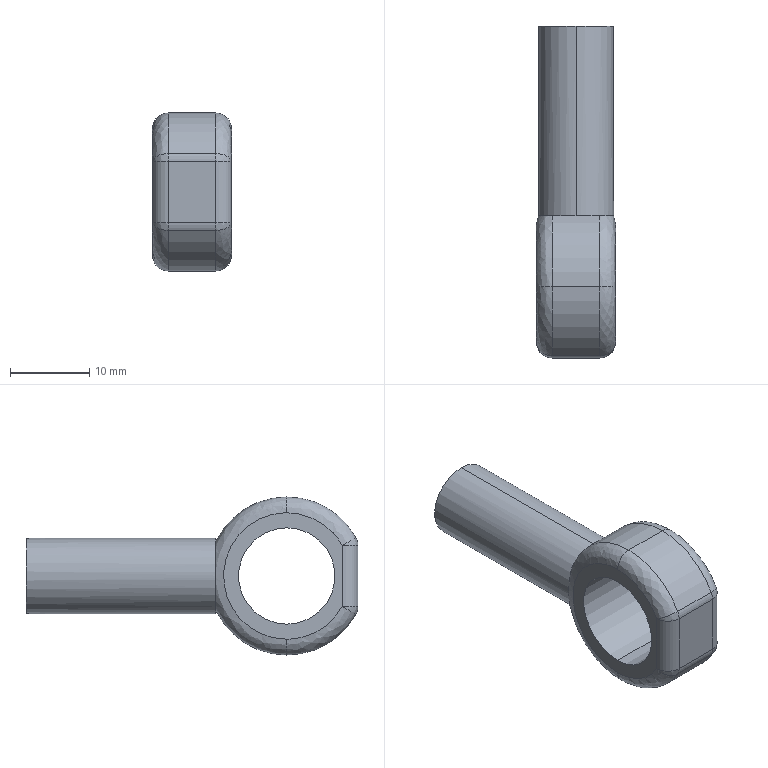Part | SolidWorks | features BaseBody 1 | 1 solid | 31 faces | box 10 x 42 x 20 mm | volume 3464 mm3 | cylinder 11 | spline 10 | plane 10 | commonest cylinder face diameters 4 x4 20 x3 9.5 x2 12.2 x2
STEP:
#1=CARTESIAN_POINT('',(5.,0.,8.));
#2=VERTEX_POINT('',#1);
#3=CARTESIAN_POINT('',(5.,-7.,3.873));
#4=VERTEX_POINT('',#3);
#5=CARTESIAN_POINT('',(5.,0.,8.));
#6=CARTESIAN_POINT('',(5.,-0.3506,8.));
#7=CARTESIAN_POINT('',(5.,-0.8722,7.966));
#8=CARTESIAN_POINT('',(5.,-1.473,7.867));
#9=CARTESIAN_POINT('',(5.,-1.771,7.802));
#10=CARTESIAN_POINT('',(5.,-1.899,7.771));
#11=CARTESIAN_POINT('',(5.,-1.984,7.75));
#12=CARTESIAN_POINT('',(5.,-2.025,7.74));
#13=CARTESIAN_POINT('',(5.,-2.771,7.54));
#14=CARTESIAN_POINT('',(5.,-3.437,7.261));
#15=CARTESIAN_POINT('',(5.,-4.376,6.707));
#16=CARTESIAN_POINT('',(5.,-4.823,6.401));
#17=CARTESIAN_POINT('',(5.,-5.305,5.993));
#18=CARTESIAN_POINT('',(5.,-5.536,5.776));
#19=CARTESIAN_POINT('',(5.,-5.633,5.681));
#20=CARTESIAN_POINT('',(5.,-5.697,5.617));
#21=CARTESIAN_POINT('',(5.,-5.73,5.583));
#22=CARTESIAN_POINT('',(5.,-6.247,5.046));
#23=CARTESIAN_POINT('',(5.,-6.66,4.487));
#24=CARTESIAN_POINT('',(5.,-7.,3.873));
#25=B_SPLINE_CURVE_WITH_KNOTS('',3,(#5,#6,#7,#8,#9,#10,#11,#12,#13,#14,#15,#16,#17,#18,#19,#20,#21,#22,#23,#24),.UNSPECIFIED.,.F.,.F.,(4,1,1,1,2,2,2,1,1,1,2,2,4),(0.,0.125,0.1875,0.2187,0.2344,0.25,0.5,0.625,0.6875,0.7187,0.7344,0.75,1.),.UNSPECIFIED.);
#26=EDGE_CURVE('',#2,#4,#25,.T.);
#27=ORIENTED_EDGE('',*,*,#26,.F.);
#28=CARTESIAN_POINT('',(3.,0.,10.));
#29=VERTEX_POINT('',#28);
#30=CARTESIAN_POINT('',(3.,0.,8.));
#31=DIRECTION('',(0.,-1.,0.));
#32=DIRECTION('',(0.,0.,1.));
#33=AXIS2_PLACEMENT_3D('',#30,#31,#32);
#34=CIRCLE('',#33,2.);
#35=EDGE_CURVE('',#2,#29,#34,.T.);
#36=ORIENTED_EDGE('',*,*,#35,.T.);
#37=CARTESIAN_POINT('',(3.,-8.75,4.841));
#38=VERTEX_POINT('',#37);
#39=CARTESIAN_POINT('',(3.,0.,0.));
#40=DIRECTION('',(1.,0.,0.));
#41=DIRECTION('',(0.,0.,-1.));
#42=AXIS2_PLACEMENT_3D('',#39,#40,#41);
#43=CIRCLE('',#42,10.);
#44=EDGE_CURVE('',#29,#38,#43,.T.);
#45=ORIENTED_EDGE('',*,*,#44,.T.);
#46=CARTESIAN_POINT('',(3.,-7.,3.873));
#47=DIRECTION('',(0.,0.4841,0.875));
#48=DIRECTION('',(0.,-0.875,0.4841));
#49=AXIS2_PLACEMENT_3D('',#46,#47,#48);
#50=CIRCLE('',#49,2.);
#51=EDGE_CURVE('',#38,#4,#50,.T.);
#52=ORIENTED_EDGE('',*,*,#51,.T.);
#53=EDGE_LOOP('',(#27,#36,#45,#52));
#54=FACE_OUTER_BOUND('',#53,.T.);
#55=CARTESIAN_POINT('',(5.,0.,8.));
#56=CARTESIAN_POINT('',(5.,-2.984,8.));
#57=CARTESIAN_POINT('',(5.,-5.555,6.484));
#58=CARTESIAN_POINT('',(5.,-7.,3.873));
#59=CARTESIAN_POINT('',(5.,0.,9.172));
#60=CARTESIAN_POINT('',(5.,-3.421,9.172));
#61=CARTESIAN_POINT('',(5.,-6.369,7.434));
#62=CARTESIAN_POINT('',(5.,-8.025,4.44));
#63=CARTESIAN_POINT('',(4.172,0.,10.));
#64=CARTESIAN_POINT('',(4.172,-3.73,10.));
#65=CARTESIAN_POINT('',(4.172,-6.944,8.105));
#66=CARTESIAN_POINT('',(4.172,-8.75,4.841));
#67=CARTESIAN_POINT('',(3.,0.,10.));
#68=CARTESIAN_POINT('',(3.,-3.73,10.));
#69=CARTESIAN_POINT('',(3.,-6.944,8.105));
#70=CARTESIAN_POINT('',(3.,-8.75,4.841));
#71=(BOUNDED_SURFACE()B_SPLINE_SURFACE(3,3,((#55,#56,#57,#58),(#59,#60,#61,#62),(#63,#64,#65,#66),(#67,#68,#69,#70)),.UNSPECIFIED.,.F.,.F.,.F.)B_SPLINE_SURFACE_WITH_KNOTS((4,4),(4,4),(0.,1.),(0.,1.),.UNSPECIFIED.)GEOMETRIC_REPRESENTATION_ITEM()RATIONAL_B_SPLINE_SURFACE(((1.,0.9076,0.9076,1.),(0.8047,0.7304,0.7304,0.8047),(0.8047,0.7304,0.7304,0.8047),(1.,0.9076,0.9076,1.)))REPRESENTATION_ITEM('')SURFACE());
#72=ADVANCED_FACE('',(#54),#71,.T.);
#73=ORIENTED_EDGE('',*,*,#35,.F.);
#74=CARTESIAN_POINT('',(5.,0.,-8.));
#75=VERTEX_POINT('',#74);
#76=CARTESIAN_POINT('',(5.,0.,8.));
#77=CARTESIAN_POINT('',(5.,16.,8.));
#78=CARTESIAN_POINT('',(5.,16.,-8.));
#79=CARTESIAN_POINT('',(5.,0.,-8.));
#80=(BOUNDED_CURVE()B_SPLINE_CURVE(3,(#76,#77,#78,#79),.UNSPECIFIED.,.F.,.T.)B_SPLINE_CURVE_WITH_KNOTS((4,4),(0.,1.),.UNSPECIFIED.)CURVE()GEOMETRIC_REPRESENTATION_ITEM()RATIONAL_B_SPLINE_CURVE((1.,0.3333,0.3333,1.))REPRESENTATION_ITEM(''));
#81=EDGE_CURVE('',#2,#75,#80,.T.);
#82=ORIENTED_EDGE('',*,*,#81,.T.);
#83=CARTESIAN_POINT('',(3.,0.,-10.));
#84=VERTEX_POINT('',#83);
#85=CARTESIAN_POINT('',(3.,0.,-8.));
#86=DIRECTION('',(0.,1.,0.));
#87=DIRECTION('',(0.,0.,-1.));
#88=AXIS2_PLACEMENT_3D('',#85,#86,#87);
#89=CIRCLE('',#88,2.);
#90=EDGE_CURVE('',#75,#84,#89,.T.);
#91=ORIENTED_EDGE('',*,*,#90,.T.);
#92=CARTESIAN_POINT('',(3.,9.,-4.359));
#93=VERTEX_POINT('',#92);
#94=CARTESIAN_POINT('',(3.,0.,0.));
#95=DIRECTION('',(-1.,0.,0.));
#96=DIRECTION('',(0.,0.,1.));
#97=AXIS2_PLACEMENT_3D('',#94,#95,#96);
#98=CIRCLE('',#97,10.);
#99=EDGE_CURVE('',#93,#84,#98,.T.);
#100=ORIENTED_EDGE('',*,*,#99,.F.);
#101=CARTESIAN_POINT('',(4.724,9.,-0.4952));
#102=VERTEX_POINT('',#101);
#103=CARTESIAN_POINT('',(3.,9.,-4.359));
#104=CARTESIAN_POINT('',(3.194,9.,-4.359));
#105=CARTESIAN_POINT('',(3.381,9.,-4.292));
#106=CARTESIAN_POINT('',(3.702,9.,-4.077));
#107=CARTESIAN_POINT('',(3.834,9.,-3.936));
#108=CARTESIAN_POINT('',(4.06,9.,-3.623));
#109=CARTESIAN_POINT('',(4.15,9.,-3.455));
#110=CARTESIAN_POINT('',(4.304,9.,-3.107));
#111=CARTESIAN_POINT('',(4.367,9.,-2.924));
#112=CARTESIAN_POINT('',(4.526,9.,-2.375));
#113=CARTESIAN_POINT('',(4.592,9.,-2.003));
#114=CARTESIAN_POINT('',(4.686,9.,-1.253));
#115=CARTESIAN_POINT('',(4.712,9.,-0.8754));
#116=CARTESIAN_POINT('',(4.724,9.,-0.4952));
#117=B_SPLINE_CURVE_WITH_KNOTS('',3,(#103,#104,#105,#106,#107,#108,#109,#110,#111,#112,#113,#114,#115,#116),.UNSPECIFIED.,.F.,.F.,(4,2,2,2,2,2,4),(0.,0.0005743,0.001149,0.001723,0.002297,0.003446,0.004594),.UNSPECIFIED.);
#118=EDGE_CURVE('',#93,#102,#117,.T.);
#119=ORIENTED_EDGE('',*,*,#118,.T.);
#120=CARTESIAN_POINT('',(4.724,9.,0.4952));
#121=VERTEX_POINT('',#120);
#122=CARTESIAN_POINT('',(4.724,9.,-0.4952));
#123=CARTESIAN_POINT('',(4.741,8.98,-0.3301));
#124=CARTESIAN_POINT('',(4.759,8.957,0.));
#125=CARTESIAN_POINT('',(4.741,8.98,0.3301));
#126=CARTESIAN_POINT('',(4.724,9.,0.4952));
#127=B_SPLINE_CURVE_WITH_KNOTS('',3,(#122,#123,#124,#125,#126),.UNSPECIFIED.,.F.,.F.,(4,1,4),(0.,0.0004952,0.0009903),.UNSPECIFIED.);
#128=EDGE_CURVE('',#102,#121,#127,.T.);
#129=ORIENTED_EDGE('',*,*,#128,.T.);
#130=CARTESIAN_POINT('',(3.,9.,4.359));
#131=VERTEX_POINT('',#130);
#132=CARTESIAN_POINT('',(4.724,9.,0.4952));
#133=CARTESIAN_POINT('',(4.712,9.,0.8759));
#134=CARTESIAN_POINT('',(4.686,9.,1.255));
#135=CARTESIAN_POINT('',(4.592,9.,2.008));
#136=CARTESIAN_POINT('',(4.524,9.,2.385));
#137=CARTESIAN_POINT('',(4.364,9.,2.934));
#138=CARTESIAN_POINT('',(4.301,9.,3.114));
#139=CARTESIAN_POINT('',(4.146,9.,3.462));
#140=CARTESIAN_POINT('',(4.056,9.,3.629));
#141=CARTESIAN_POINT('',(3.835,9.,3.936));
#142=CARTESIAN_POINT('',(3.701,9.,4.079));
#143=CARTESIAN_POINT('',(3.461,9.,4.239));
#144=CARTESIAN_POINT('',(3.374,9.,4.282));
#145=CARTESIAN_POINT('',(3.194,9.,4.342));
#146=CARTESIAN_POINT('',(3.097,9.,4.359));
#147=CARTESIAN_POINT('',(3.,9.,4.359));
#148=B_SPLINE_CURVE_WITH_KNOTS('',3,(#132,#133,#134,#135,#136,#137,#138,#139,#140,#141,#142,#143,#144,#145,#146,#147),.UNSPECIFIED.,.F.,.F.,(4,2,2,2,2,2,2,4),(0.,0.001139,0.002277,0.002846,0.003416,0.003985,0.00427,0.004554),.UNSPECIFIED.);
#149=EDGE_CURVE('',#121,#131,#148,.T.);
#150=ORIENTED_EDGE('',*,*,#149,.T.);
#151=CARTESIAN_POINT('',(3.,0.,0.));
#152=DIRECTION('',(1.,0.,0.));
#153=DIRECTION('',(0.,0.,-1.));
#154=AXIS2_PLACEMENT_3D('',#151,#152,#153);
#155=CIRCLE('',#154,10.);
#156=EDGE_CURVE('',#131,#29,#155,.T.);
#157=ORIENTED_EDGE('',*,*,#156,.T.);
#158=EDGE_LOOP('',(#73,#82,#91,#100,#119,#129,#150,#157));
#159=FACE_OUTER_BOUND('',#158,.T.);
#160=CARTESIAN_POINT('',(5.,0.,-8.));
#161=CARTESIAN_POINT('',(5.,16.,-8.));
#162=CARTESIAN_POINT('',(5.,16.,8.));
#163=CARTESIAN_POINT('',(5.,0.,8.));
#164=CARTESIAN_POINT('',(5.,0.,-9.172));
#165=CARTESIAN_POINT('',(5.,18.343,-9.172));
#166=CARTESIAN_POINT('',(5.,18.343,9.172));
#167=CARTESIAN_POINT('',(5.,0.,9.172));
#168=CARTESIAN_POINT('',(4.172,0.,-10.));
#169=CARTESIAN_POINT('',(4.172,20.,-10.));
#170=CARTESIAN_POINT('',(4.172,20.,10.));
#171=CARTESIAN_POINT('',(4.172,0.,10.));
#172=CARTESIAN_POINT('',(3.,0.,-10.));
#173=CARTESIAN_POINT('',(3.,20.,-10.));
#174=CARTESIAN_POINT('',(3.,20.,10.));
#175=CARTESIAN_POINT('',(3.,0.,10.));
#176=(BOUNDED_SURFACE()B_SPLINE_SURFACE(3,3,((#160,#161,#162,#163),(#164,#165,#166,#167),(#168,#169,#170,#171),(#172,#173,#174,#175)),.UNSPECIFIED.,.F.,.F.,.F.)B_SPLINE_SURFACE_WITH_KNOTS((4,4),(4,4),(0.,1.),(0.,1.),.UNSPECIFIED.)GEOMETRIC_REPRESENTATION_ITEM()RATIONAL_B_SPLINE_SURFACE(((1.,0.3333,0.3333,1.),(0.8047,0.2682,0.2682,0.8047),(0.8047,0.2682,0.2682,0.8047),(1.,0.3333,0.3333,1.)))REPRESENTATION_ITEM('')SURFACE());
#177=ADVANCED_FACE('',(#159),#176,.T.);
#178=CARTESIAN_POINT('',(-3.,0.,10.));
#179=VERTEX_POINT('',#178);
#180=CARTESIAN_POINT('',(-3.,-8.75,4.841));
#181=VERTEX_POINT('',#180);
#182=CARTESIAN_POINT('',(-3.,0.,0.));
#183=DIRECTION('',(1.,0.,0.));
#184=DIRECTION('',(0.,0.,1.));
#185=AXIS2_PLACEMENT_3D('',#182,#183,#184);
#186=CIRCLE('',#185,10.);
#187=EDGE_CURVE('',#179,#181,#186,.T.);
#188=ORIENTED_EDGE('',*,*,#187,.F.);
#189=CARTESIAN_POINT('',(-5.,0.,8.));
#190=VERTEX_POINT('',#189);
#191=CARTESIAN_POINT('',(-3.,0.,8.));
#192=DIRECTION('',(0.,-1.,0.));
#193=DIRECTION('',(0.,0.,1.));
#194=AXIS2_PLACEMENT_3D('',#191,#192,#193);
#195=CIRCLE('',#194,2.);
#196=EDGE_CURVE('',#179,#190,#195,.T.);
#197=ORIENTED_EDGE('',*,*,#196,.T.);
#198=CARTESIAN_POINT('',(-5.,-7.,3.873));
#199=VERTEX_POINT('',#198);
#200=CARTESIAN_POINT('',(-5.,0.,8.));
#201=CARTESIAN_POINT('',(-5.,-2.984,8.));
#202=CARTESIAN_POINT('',(-5.,-5.555,6.484));
#203=CARTESIAN_POINT('',(-5.,-7.,3.873));
#204=(BOUNDED_CURVE()B_SPLINE_CURVE(3,(#200,#201,#202,#203),.UNSPECIFIED.,.F.,.F.)B_SPLINE_CURVE_WITH_KNOTS((4,4),(0.,1.),.UNSPECIFIED.)CURVE()GEOMETRIC_REPRESENTATION_ITEM()RATIONAL_B_SPLINE_CURVE((1.,0.9076,0.9076,1.))REPRESENTATION_ITEM(''));
#205=EDGE_CURVE('',#190,#199,#204,.T.);
#206=ORIENTED_EDGE('',*,*,#205,.T.);
#207=CARTESIAN_POINT('',(-3.,-7.,3.873));
#208=DIRECTION('',(0.,0.4841,0.875));
#209=DIRECTION('',(0.,-0.875,0.4841));
#210=AXIS2_PLACEMENT_3D('',#207,#208,#209);
#211=CIRCLE('',#210,2.);
#212=EDGE_CURVE('',#199,#181,#211,.T.);
#213=ORIENTED_EDGE('',*,*,#212,.T.);
#214=EDGE_LOOP('',(#188,#197,#206,#213));
#215=FACE_OUTER_BOUND('',#214,.T.);
#216=CARTESIAN_POINT('',(-3.,0.,10.));
#217=CARTESIAN_POINT('',(-3.,-3.73,10.));
#218=CARTESIAN_POINT('',(-3.,-6.944,8.105));
#219=CARTESIAN_POINT('',(-3.,-8.75,4.841));
#220=CARTESIAN_POINT('',(-4.172,0.,10.));
#221=CARTESIAN_POINT('',(-4.172,-3.73,10.));
#222=CARTESIAN_POINT('',(-4.172,-6.944,8.105));
#223=CARTESIAN_POINT('',(-4.172,-8.75,4.841));
#224=CARTESIAN_POINT('',(-5.,0.,9.172));
#225=CARTESIAN_POINT('',(-5.,-3.421,9.172));
#226=CARTESIAN_POINT('',(-5.,-6.369,7.434));
#227=CARTESIAN_POINT('',(-5.,-8.025,4.44));
#228=CARTESIAN_POINT('',(-5.,0.,8.));
#229=CARTESIAN_POINT('',(-5.,-2.984,8.));
#230=CARTESIAN_POINT('',(-5.,-5.555,6.484));
#231=CARTESIAN_POINT('',(-5.,-7.,3.873));
#232=(BOUNDED_SURFACE()B_SPLINE_SURFACE(3,3,((#216,#217,#218,#219),(#220,#221,#222,#223),(#224,#225,#226,#227),(#228,#229,#230,#231)),.UNSPECIFIED.,.F.,.F.,.F.)B_SPLINE_SURFACE_WITH_KNOTS((4,4),(4,4),(0.,1.),(0.,1.),.UNSPECIFIED.)GEOMETRIC_REPRESENTATION_ITEM()RATIONAL_B_SPLINE_SURFACE(((1.,0.9076,0.9076,1.),(0.8047,0.7304,0.7304,0.8047),(0.8047,0.7304,0.7304,0.8047),(1.,0.9076,0.9076,1.)))REPRESENTATION_ITEM('')SURFACE());
#233=ADVANCED_FACE('',(#215),#232,.T.);
#234=ORIENTED_EDGE('',*,*,#196,.F.);
#235=CARTESIAN_POINT('',(-3.,9.,4.359));
#236=VERTEX_POINT('',#235);
#237=CARTESIAN_POINT('',(-3.,0.,0.));
#238=DIRECTION('',(1.,0.,0.));
#239=DIRECTION('',(0.,0.,1.));
#240=AXIS2_PLACEMENT_3D('',#237,#238,#239);
#241=CIRCLE('',#240,10.);
#242=EDGE_CURVE('',#236,#179,#241,.T.);
#243=ORIENTED_EDGE('',*,*,#242,.F.);
#244=CARTESIAN_POINT('',(-4.724,9.,0.4952));
#245=VERTEX_POINT('',#244);
#246=CARTESIAN_POINT('',(-3.,9.,4.359));
#247=CARTESIAN_POINT('',(-3.194,9.,4.359));
#248=CARTESIAN_POINT('',(-3.381,9.,4.292));
#249=CARTESIAN_POINT('',(-3.702,9.,4.077));
#250=CARTESIAN_POINT('',(-3.834,9.,3.936));
#251=CARTESIAN_POINT('',(-4.06,9.,3.623));
#252=CARTESIAN_POINT('',(-4.15,9.,3.455));
#253=CARTESIAN_POINT('',(-4.304,9.,3.107));
#254=CARTESIAN_POINT('',(-4.367,9.,2.924));
#255=CARTESIAN_POINT('',(-4.526,9.,2.375));
#256=CARTESIAN_POINT('',(-4.592,9.,2.003));
#257=CARTESIAN_POINT('',(-4.686,9.,1.253));
#258=CARTESIAN_POINT('',(-4.712,9.,0.8754));
#259=CARTESIAN_POINT('',(-4.724,9.,0.4952));
#260=B_SPLINE_CURVE_WITH_KNOTS('',3,(#246,#247,#248,#249,#250,#251,#252,#253,#254,#255,#256,#257,#258,#259),.UNSPECIFIED.,.F.,.F.,(4,2,2,2,2,2,4),(0.,0.0005743,0.001149,0.001723,0.002297,0.003446,0.004594),.UNSPECIFIED.);
#261=EDGE_CURVE('',#236,#245,#260,.T.);
#262=ORIENTED_EDGE('',*,*,#261,.T.);
#263=CARTESIAN_POINT('',(-4.724,9.,-0.4952));
#264=VERTEX_POINT('',#263);
#265=CARTESIAN_POINT('',(-4.724,9.,0.4952));
#266=CARTESIAN_POINT('',(-4.741,8.98,0.3301));
#267=CARTESIAN_POINT('',(-4.759,8.957,0.));
#268=CARTESIAN_POINT('',(-4.741,8.98,-0.3301));
#269=CARTESIAN_POINT('',(-4.724,9.,-0.4952));
#270=B_SPLINE_CURVE_WITH_KNOTS('',3,(#265,#266,#267,#268,#269),.UNSPECIFIED.,.F.,.F.,(4,1,4),(0.,0.0004952,0.0009903),.UNSPECIFIED.);
#271=EDGE_CURVE('',#245,#264,#270,.T.);
#272=ORIENTED_EDGE('',*,*,#271,.T.);
#273=CARTESIAN_POINT('',(-3.,9.,-4.359));
#274=VERTEX_POINT('',#273);
#275=CARTESIAN_POINT('',(-4.724,9.,-0.4952));
#276=CARTESIAN_POINT('',(-4.712,9.,-0.8759));
#277=CARTESIAN_POINT('',(-4.686,9.,-1.255));
#278=CARTESIAN_POINT('',(-4.592,9.,-2.008));
#279=CARTESIAN_POINT('',(-4.524,9.,-2.385));
#280=CARTESIAN_POINT('',(-4.364,9.,-2.934));
#281=CARTESIAN_POINT('',(-4.301,9.,-3.114));
#282=CARTESIAN_POINT('',(-4.146,9.,-3.462));
#283=CARTESIAN_POINT('',(-4.056,9.,-3.629));
#284=CARTESIAN_POINT('',(-3.835,9.,-3.936));
#285=CARTESIAN_POINT('',(-3.701,9.,-4.079));
#286=CARTESIAN_POINT('',(-3.461,9.,-4.239));
#287=CARTESIAN_POINT('',(-3.374,9.,-4.282));
#288=CARTESIAN_POINT('',(-3.194,9.,-4.342));
#289=CARTESIAN_POINT('',(-3.097,9.,-4.359));
#290=CARTESIAN_POINT('',(-3.,9.,-4.359));
#291=B_SPLINE_CURVE_WITH_KNOTS('',3,(#275,#276,#277,#278,#279,#280,#281,#282,#283,#284,#285,#286,#287,#288,#289,#290),.UNSPECIFIED.,.F.,.F.,(4,2,2,2,2,2,2,4),(0.,0.001139,0.002277,0.002846,0.003416,0.003985,0.00427,0.004554),.UNSPECIFIED.);
#292=EDGE_CURVE('',#264,#274,#291,.T.);
#293=ORIENTED_EDGE('',*,*,#292,.T.);
#294=CARTESIAN_POINT('',(-3.,0.,-10.));
#295=VERTEX_POINT('',#294);
#296=CARTESIAN_POINT('',(-3.,0.,0.));
#297=DIRECTION('',(1.,0.,0.));
#298=DIRECTION('',(0.,0.,1.));
#299=AXIS2_PLACEMENT_3D('',#296,#297,#298);
#300=CIRCLE('',#299,10.);
#301=EDGE_CURVE('',#295,#274,#300,.T.);
#302=ORIENTED_EDGE('',*,*,#301,.F.);
#303=CARTESIAN_POINT('',(-5.,0.,-8.));
#304=VERTEX_POINT('',#303);
#305=CARTESIAN_POINT('',(-3.,0.,-8.));
#306=DIRECTION('',(0.,1.,0.));
#307=DIRECTION('',(0.,0.,-1.));
#308=AXIS2_PLACEMENT_3D('',#305,#306,#307);
#309=CIRCLE('',#308,2.);
#310=EDGE_CURVE('',#295,#304,#309,.T.);
#311=ORIENTED_EDGE('',*,*,#310,.T.);
#312=CARTESIAN_POINT('',(-5.,0.,-8.));
#313=CARTESIAN_POINT('',(-5.,16.,-8.));
#314=CARTESIAN_POINT('',(-5.,16.,8.));
#315=CARTESIAN_POINT('',(-5.,0.,8.));
#316=(BOUNDED_CURVE()B_SPLINE_CURVE(3,(#312,#313,#314,#315),.UNSPECIFIED.,.F.,.F.)B_SPLINE_CURVE_WITH_KNOTS((4,4),(0.,1.),.UNSPECIFIED.)CURVE()GEOMETRIC_REPRESENTATION_ITEM()RATIONAL_B_SPLINE_CURVE((1.,0.3333,0.3333,1.))REPRESENTATION_ITEM(''));
#317=EDGE_CURVE('',#304,#190,#316,.T.);
#318=ORIENTED_EDGE('',*,*,#317,.T.);
#319=EDGE_LOOP('',(#234,#243,#262,#272,#293,#302,#311,#318));
#320=FACE_OUTER_BOUND('',#319,.T.);
#321=CARTESIAN_POINT('',(-3.,0.,-10.));
#322=CARTESIAN_POINT('',(-3.,20.,-10.));
#323=CARTESIAN_POINT('',(-3.,20.,10.));
#324=CARTESIAN_POINT('',(-3.,0.,10.));
#325=CARTESIAN_POINT('',(-4.172,0.,-10.));
#326=CARTESIAN_POINT('',(-4.172,20.,-10.));
#327=CARTESIAN_POINT('',(-4.172,20.,10.));
#328=CARTESIAN_POINT('',(-4.172,0.,10.));
#329=CARTESIAN_POINT('',(-5.,0.,-9.172));
#330=CARTESIAN_POINT('',(-5.,18.343,-9.172));
#331=CARTESIAN_POINT('',(-5.,18.343,9.172));
#332=CARTESIAN_POINT('',(-5.,0.,9.172));
#333=CARTESIAN_POINT('',(-5.,0.,-8.));
#334=CARTESIAN_POINT('',(-5.,16.,-8.));
#335=CARTESIAN_POINT('',(-5.,16.,8.));
#336=CARTESIAN_POINT('',(-5.,0.,8.));
#337=(BOUNDED_SURFACE()B_SPLINE_SURFACE(3,3,((#321,#322,#323,#324),(#325,#326,#327,#328),(#329,#330,#331,#332),(#333,#334,#335,#336)),.UNSPECIFIED.,.F.,.F.,.T.)B_SPLINE_SURFACE_WITH_KNOTS((4,4),(4,4),(0.,1.),(0.,1.),.UNSPECIFIED.)GEOMETRIC_REPRESENTATION_ITEM()RATIONAL_B_SPLINE_SURFACE(((1.,0.3333,0.3333,1.),(0.8047,0.2682,0.2682,0.8047),(0.8047,0.2682,0.2682,0.8047),(1.,0.3333,0.3333,1.)))REPRESENTATION_ITEM('')SURFACE());
#338=ADVANCED_FACE('',(#320),#337,.T.);
#339=CARTESIAN_POINT('',(0.,33.,-4.75));
#340=VERTEX_POINT('',#339);
#341=CARTESIAN_POINT('',(0.,33.,4.75));
#342=VERTEX_POINT('',#341);
#343=CARTESIAN_POINT('',(0.,33.,0.));
#344=DIRECTION('',(0.,-1.,0.));
#345=DIRECTION('',(0.,0.,-1.));
#346=AXIS2_PLACEMENT_3D('',#343,#344,#345);
#347=CIRCLE('',#346,4.75);
#348=EDGE_CURVE('',#340,#342,#347,.T.);
#349=ORIENTED_EDGE('',*,*,#348,.T.);
#350=CARTESIAN_POINT('',(0.,9.,4.75));
#351=VERTEX_POINT('',#350);
#352=CARTESIAN_POINT('',(0.,33.,4.75));
#353=DIRECTION('',(0.,-1.,0.));
#354=VECTOR('',#353,1000.);
#355=LINE('',#352,#354);
#356=EDGE_CURVE('',#342,#351,#355,.T.);
#357=ORIENTED_EDGE('',*,*,#356,.T.);
#358=CARTESIAN_POINT('',(1.887,9.,4.359));
#359=VERTEX_POINT('',#358);
#360=CARTESIAN_POINT('',(0.,9.,0.));
#361=DIRECTION('',(0.,1.,0.));
#362=DIRECTION('',(0.,0.,-1.));
#363=AXIS2_PLACEMENT_3D('',#360,#361,#362);
#364=CIRCLE('',#363,4.75);
#365=EDGE_CURVE('',#351,#359,#364,.T.);
#366=ORIENTED_EDGE('',*,*,#365,.T.);
#367=CARTESIAN_POINT('',(0.,9.,0.));
#368=DIRECTION('',(0.,1.,0.));
#369=DIRECTION('',(0.,0.,-1.));
#370=AXIS2_PLACEMENT_3D('',#367,#368,#369);
#371=CIRCLE('',#370,4.75);
#372=EDGE_CURVE('',#359,#121,#371,.T.);
#373=ORIENTED_EDGE('',*,*,#372,.T.);
#374=ORIENTED_EDGE('',*,*,#128,.F.);
#375=CARTESIAN_POINT('',(1.887,9.,-4.359));
#376=VERTEX_POINT('',#375);
#377=CARTESIAN_POINT('',(0.,9.,0.));
#378=DIRECTION('',(0.,1.,0.));
#379=DIRECTION('',(0.,0.,-1.));
#380=AXIS2_PLACEMENT_3D('',#377,#378,#379);
#381=CIRCLE('',#380,4.75);
#382=EDGE_CURVE('',#102,#376,#381,.T.);
#383=ORIENTED_EDGE('',*,*,#382,.T.);
#384=CARTESIAN_POINT('',(0.,9.,-4.75));
#385=VERTEX_POINT('',#384);
#386=CARTESIAN_POINT('',(0.,9.,0.));
#387=DIRECTION('',(0.,1.,0.));
#388=DIRECTION('',(0.,0.,-1.));
#389=AXIS2_PLACEMENT_3D('',#386,#387,#388);
#390=CIRCLE('',#389,4.75);
#391=EDGE_CURVE('',#376,#385,#390,.T.);
#392=ORIENTED_EDGE('',*,*,#391,.T.);
#393=CARTESIAN_POINT('',(0.,33.,-4.75));
#394=DIRECTION('',(0.,-1.,0.));
#395=VECTOR('',#394,1000.);
#396=LINE('',#393,#395);
#397=EDGE_CURVE('',#340,#385,#396,.T.);
#398=ORIENTED_EDGE('',*,*,#397,.F.);
#399=EDGE_LOOP('',(#349,#357,#366,#373,#374,#383,#392,#398));
#400=FACE_OUTER_BOUND('',#399,.T.);
#401=CARTESIAN_POINT('',(0.,33.,0.));
#402=DIRECTION('',(0.,-1.,0.));
#403=DIRECTION('',(0.,0.,-1.));
#404=AXIS2_PLACEMENT_3D('',#401,#402,#403);
#405=CYLINDRICAL_SURFACE('',#404,4.75);
#406=ADVANCED_FACE('',(#400),#405,.T.);
#407=ORIENTED_EDGE('',*,*,#44,.F.);
#408=CARTESIAN_POINT('',(5.,0.,10.));
#409=DIRECTION('',(-1.,0.,0.));
#410=VECTOR('',#409,1000.);
#411=LINE('',#408,#410);
#412=EDGE_CURVE('',#29,#179,#411,.T.);
#413=ORIENTED_EDGE('',*,*,#412,.T.);
#414=ORIENTED_EDGE('',*,*,#187,.T.);
#415=CARTESIAN_POINT('',(5.,-8.75,4.841));
#416=DIRECTION('',(1.,0.,0.));
#417=VECTOR('',#416,1000.);
#418=LINE('',#415,#417);
#419=EDGE_CURVE('',#181,#38,#418,.T.);
#420=ORIENTED_EDGE('',*,*,#419,.T.);
#421=EDGE_LOOP('',(#407,#413,#414,#420));
#422=FACE_OUTER_BOUND('',#421,.T.);
#423=CARTESIAN_POINT('',(5.,0.,0.));
#424=DIRECTION('',(-1.,0.,0.));
#425=DIRECTION('',(0.,0.,1.));
#426=AXIS2_PLACEMENT_3D('',#423,#424,#425);
#427=CYLINDRICAL_SURFACE('',#426,10.);
#428=ADVANCED_FACE('',(#422),#427,.T.);
#429=CARTESIAN_POINT('',(5.,0.,-6.1));
#430=VERTEX_POINT('',#429);
#431=CARTESIAN_POINT('',(5.,0.,6.1));
#432=VERTEX_POINT('',#431);
#433=CARTESIAN_POINT('',(5.,0.,0.));
#434=DIRECTION('',(-1.,0.,0.));
#435=DIRECTION('',(0.,0.,1.));
#436=AXIS2_PLACEMENT_3D('',#433,#434,#435);
#437=CIRCLE('',#436,6.1);
#438=EDGE_CURVE('',#430,#432,#437,.T.);
#439=ORIENTED_EDGE('',*,*,#438,.F.);
#440=CARTESIAN_POINT('',(-5.,0.,-6.1));
#441=VERTEX_POINT('',#440);
#442=CARTESIAN_POINT('',(5.,0.,-6.1));
#443=DIRECTION('',(-1.,0.,0.));
#444=VECTOR('',#443,1000.);
#445=LINE('',#442,#444);
#446=EDGE_CURVE('',#430,#441,#445,.T.);
#447=ORIENTED_EDGE('',*,*,#446,.T.);
#448=CARTESIAN_POINT('',(-5.,0.,6.1));
#449=VERTEX_POINT('',#448);
#450=CARTESIAN_POINT('',(-5.,0.,0.));
#451=DIRECTION('',(-1.,0.,0.));
#452=DIRECTION('',(0.,0.,1.));
#453=AXIS2_PLACEMENT_3D('',#450,#451,#452);
#454=CIRCLE('',#453,6.1);
#455=EDGE_CURVE('',#441,#449,#454,.T.);
#456=ORIENTED_EDGE('',*,*,#455,.T.);
#457=CARTESIAN_POINT('',(5.,0.,6.1));
#458=DIRECTION('',(-1.,0.,0.));
#459=VECTOR('',#458,1000.);
#460=LINE('',#457,#459);
#461=EDGE_CURVE('',#432,#449,#460,.T.);
#462=ORIENTED_EDGE('',*,*,#461,.F.);
#463=EDGE_LOOP('',(#439,#447,#456,#462));
#464=FACE_OUTER_BOUND('',#463,.T.);
#465=CARTESIAN_POINT('',(5.,0.,0.));
#466=DIRECTION('',(-1.,0.,0.));
#467=DIRECTION('',(0.,0.,1.));
#468=AXIS2_PLACEMENT_3D('',#465,#466,#467);
#469=CYLINDRICAL_SURFACE('',#468,6.1);
#470=ADVANCED_FACE('',(#464),#469,.F.);
#471=ORIENTED_EDGE('',*,*,#356,.F.);
#472=CARTESIAN_POINT('',(0.,33.,0.));
#473=DIRECTION('',(0.,-1.,0.));
#474=DIRECTION('',(0.,0.,-1.));
#475=AXIS2_PLACEMENT_3D('',#472,#473,#474);
#476=CIRCLE('',#475,4.75);
#477=EDGE_CURVE('',#342,#340,#476,.T.);
#478=ORIENTED_EDGE('',*,*,#477,.T.);
#479=ORIENTED_EDGE('',*,*,#397,.T.);
#480=CARTESIAN_POINT('',(-1.887,9.,-4.359));
#481=VERTEX_POINT('',#480);
#482=CARTESIAN_POINT('',(0.,9.,0.));
#483=DIRECTION('',(0.,1.,0.));
#484=DIRECTION('',(0.,0.,-1.));
#485=AXIS2_PLACEMENT_3D('',#482,#483,#484);
#486=CIRCLE('',#485,4.75);
#487=EDGE_CURVE('',#385,#481,#486,.T.);
#488=ORIENTED_EDGE('',*,*,#487,.T.);
#489=CARTESIAN_POINT('',(0.,9.,0.));
#490=DIRECTION('',(0.,1.,0.));
#491=DIRECTION('',(0.,0.,-1.));
#492=AXIS2_PLACEMENT_3D('',#489,#490,#491);
#493=CIRCLE('',#492,4.75);
#494=EDGE_CURVE('',#481,#264,#493,.T.);
#495=ORIENTED_EDGE('',*,*,#494,.T.);
#496=ORIENTED_EDGE('',*,*,#271,.F.);
#497=CARTESIAN_POINT('',(-1.887,9.,4.359));
#498=VERTEX_POINT('',#497);
#499=CARTESIAN_POINT('',(0.,9.,0.));
#500=DIRECTION('',(0.,1.,0.));
#501=DIRECTION('',(0.,0.,-1.));
#502=AXIS2_PLACEMENT_3D('',#499,#500,#501);
#503=CIRCLE('',#502,4.75);
#504=EDGE_CURVE('',#245,#498,#503,.T.);
#505=ORIENTED_EDGE('',*,*,#504,.T.);
#506=CARTESIAN_POINT('',(0.,9.,0.));
#507=DIRECTION('',(0.,1.,0.));
#508=DIRECTION('',(0.,0.,-1.));
#509=AXIS2_PLACEMENT_3D('',#506,#507,#508);
#510=CIRCLE('',#509,4.75);
#511=EDGE_CURVE('',#498,#351,#510,.T.);
#512=ORIENTED_EDGE('',*,*,#511,.T.);
#513=EDGE_LOOP('',(#471,#478,#479,#488,#495,#496,#505,#512));
#514=FACE_OUTER_BOUND('',#513,.T.);
#515=CARTESIAN_POINT('',(0.,33.,0.));
#516=DIRECTION('',(0.,-1.,0.));
#517=DIRECTION('',(0.,0.,-1.));
#518=AXIS2_PLACEMENT_3D('',#515,#516,#517);
#519=CYLINDRICAL_SURFACE('',#518,4.75);
#520=ADVANCED_FACE('',(#514),#519,.T.);
#521=CARTESIAN_POINT('',(0.,9.,-4.359));
#522=DIRECTION('',(1.,0.,0.));
#523=VECTOR('',#522,1000.);
#524=LINE('',#521,#523);
#525=EDGE_CURVE('',#481,#376,#524,.T.);
#526=ORIENTED_EDGE('',*,*,#525,.F.);
#527=ORIENTED_EDGE('',*,*,#487,.F.);
#528=ORIENTED_EDGE('',*,*,#391,.F.);
#529=EDGE_LOOP('',(#526,#527,#528));
#530=FACE_OUTER_BOUND('',#529,.T.);
#531=CARTESIAN_POINT('',(0.,9.,0.));
#532=DIRECTION('',(0.,1.,0.));
#533=DIRECTION('',(0.,0.,1.));
#534=AXIS2_PLACEMENT_3D('',#531,#532,#533);
#535=PLANE('',#534);
#536=ADVANCED_FACE('',(#530),#535,.F.);
#537=ORIENTED_EDGE('',*,*,#118,.F.);
#538=CARTESIAN_POINT('',(5.,9.,-4.359));
#539=DIRECTION('',(1.,0.,0.));
#540=VECTOR('',#539,1000.);
#541=LINE('',#538,#540);
#542=EDGE_CURVE('',#376,#93,#541,.T.);
#543=ORIENTED_EDGE('',*,*,#542,.F.);
#544=ORIENTED_EDGE('',*,*,#382,.F.);
#545=EDGE_LOOP('',(#537,#543,#544));
#546=FACE_OUTER_BOUND('',#545,.T.);
#547=CARTESIAN_POINT('',(5.,9.,4.359));
#548=DIRECTION('',(0.,-1.,0.));
#549=DIRECTION('',(0.,0.,-1.));
#550=AXIS2_PLACEMENT_3D('',#547,#548,#549);
#551=PLANE('',#550);
#552=ADVANCED_FACE('',(#546),#551,.F.);
#553=CARTESIAN_POINT('',(5.,9.,4.359));
#554=DIRECTION('',(-1.,0.,0.));
#555=VECTOR('',#554,1000.);
#556=LINE('',#553,#555);
#557=EDGE_CURVE('',#131,#359,#556,.T.);
#558=ORIENTED_EDGE('',*,*,#557,.F.);
#559=ORIENTED_EDGE('',*,*,#149,.F.);
#560=ORIENTED_EDGE('',*,*,#372,.F.);
#561=EDGE_LOOP('',(#558,#559,#560));
#562=FACE_OUTER_BOUND('',#561,.T.);
#563=CARTESIAN_POINT('',(5.,9.,4.359));
#564=DIRECTION('',(0.,-1.,0.));
#565=DIRECTION('',(0.,0.,-1.));
#566=AXIS2_PLACEMENT_3D('',#563,#564,#565);
#567=PLANE('',#566);
#568=ADVANCED_FACE('',(#562),#567,.F.);
#569=CARTESIAN_POINT('',(0.,9.,4.359));
#570=DIRECTION('',(-1.,0.,0.));
#571=VECTOR('',#570,1000.);
#572=LINE('',#569,#571);
#573=EDGE_CURVE('',#359,#498,#572,.T.);
#574=ORIENTED_EDGE('',*,*,#573,.F.);
#575=ORIENTED_EDGE('',*,*,#365,.F.);
#576=ORIENTED_EDGE('',*,*,#511,.F.);
#577=EDGE_LOOP('',(#574,#575,#576));
#578=FACE_OUTER_BOUND('',#577,.T.);
#579=CARTESIAN_POINT('',(0.,9.,0.));
#580=DIRECTION('',(0.,1.,0.));
#581=DIRECTION('',(0.,0.,1.));
#582=AXIS2_PLACEMENT_3D('',#579,#580,#581);
#583=PLANE('',#582);
#584=ADVANCED_FACE('',(#578),#583,.F.);
#585=ORIENTED_EDGE('',*,*,#348,.F.);
#586=ORIENTED_EDGE('',*,*,#477,.F.);
#587=EDGE_LOOP('',(#585,#586));
#588=FACE_OUTER_BOUND('',#587,.T.);
#589=CARTESIAN_POINT('',(0.,33.,0.));
#590=DIRECTION('',(0.,1.,0.));
#591=DIRECTION('',(0.,0.,1.));
#592=AXIS2_PLACEMENT_3D('',#589,#590,#591);
#593=PLANE('',#592);
#594=ADVANCED_FACE('',(#588),#593,.T.);
#595=ORIENTED_EDGE('',*,*,#261,.F.);
#596=CARTESIAN_POINT('',(5.,9.,4.359));
#597=DIRECTION('',(-1.,0.,0.));
#598=VECTOR('',#597,1000.);
#599=LINE('',#596,#598);
#600=EDGE_CURVE('',#498,#236,#599,.T.);
#601=ORIENTED_EDGE('',*,*,#600,.F.);
#602=ORIENTED_EDGE('',*,*,#504,.F.);
#603=EDGE_LOOP('',(#595,#601,#602));
#604=FACE_OUTER_BOUND('',#603,.T.);
#605=CARTESIAN_POINT('',(5.,9.,4.359));
#606=DIRECTION('',(0.,-1.,0.));
#607=DIRECTION('',(0.,0.,-1.));
#608=AXIS2_PLACEMENT_3D('',#605,#606,#607);
#609=PLANE('',#608);
#610=ADVANCED_FACE('',(#604),#609,.F.);
#611=CARTESIAN_POINT('',(5.,9.,-4.359));
#612=DIRECTION('',(1.,0.,0.));
#613=VECTOR('',#612,1000.);
#614=LINE('',#611,#613);
#615=EDGE_CURVE('',#274,#481,#614,.T.);
#616=ORIENTED_EDGE('',*,*,#615,.F.);
#617=ORIENTED_EDGE('',*,*,#292,.F.);
#618=ORIENTED_EDGE('',*,*,#494,.F.);
#619=EDGE_LOOP('',(#616,#617,#618));
#620=FACE_OUTER_BOUND('',#619,.T.);
#621=CARTESIAN_POINT('',(5.,9.,4.359));
#622=DIRECTION('',(0.,-1.,0.));
#623=DIRECTION('',(0.,0.,-1.));
#624=AXIS2_PLACEMENT_3D('',#621,#622,#623);
#625=PLANE('',#624);
#626=ADVANCED_FACE('',(#620),#625,.F.);
#627=ORIENTED_EDGE('',*,*,#525,.T.);
#628=ORIENTED_EDGE('',*,*,#542,.T.);
#629=ORIENTED_EDGE('',*,*,#99,.T.);
#630=CARTESIAN_POINT('',(3.,-8.75,-4.841));
#631=VERTEX_POINT('',#630);
#632=CARTESIAN_POINT('',(3.,0.,0.));
#633=DIRECTION('',(-1.,0.,0.));
#634=DIRECTION('',(0.,0.,1.));
#635=AXIS2_PLACEMENT_3D('',#632,#633,#634);
#636=CIRCLE('',#635,10.);
#637=EDGE_CURVE('',#84,#631,#636,.T.);
#638=ORIENTED_EDGE('',*,*,#637,.T.);
#639=CARTESIAN_POINT('',(-3.,-8.75,-4.841));
#640=VERTEX_POINT('',#639);
#641=CARTESIAN_POINT('',(5.,-8.75,-4.841));
#642=DIRECTION('',(-1.,0.,0.));
#643=VECTOR('',#642,1000.);
#644=LINE('',#641,#643);
#645=EDGE_CURVE('',#631,#640,#644,.T.);
#646=ORIENTED_EDGE('',*,*,#645,.T.);
#647=CARTESIAN_POINT('',(-3.,0.,0.));
#648=DIRECTION('',(1.,0.,0.));
#649=DIRECTION('',(0.,0.,1.));
#650=AXIS2_PLACEMENT_3D('',#647,#648,#649);
#651=CIRCLE('',#650,10.);
#652=EDGE_CURVE('',#640,#295,#651,.T.);
#653=ORIENTED_EDGE('',*,*,#652,.T.);
#654=ORIENTED_EDGE('',*,*,#301,.T.);
#655=ORIENTED_EDGE('',*,*,#615,.T.);
#656=EDGE_LOOP('',(#627,#628,#629,#638,#646,#653,#654,#655));
#657=FACE_OUTER_BOUND('',#656,.T.);
#658=CARTESIAN_POINT('',(5.,0.,0.));
#659=DIRECTION('',(-1.,0.,0.));
#660=DIRECTION('',(0.,0.,1.));
#661=AXIS2_PLACEMENT_3D('',#658,#659,#660);
#662=CYLINDRICAL_SURFACE('',#661,10.);
#663=ADVANCED_FACE('',(#657),#662,.T.);
#664=ORIENTED_EDGE('',*,*,#90,.F.);
#665=CARTESIAN_POINT('',(5.,-7.,-3.873));
#666=VERTEX_POINT('',#665);
#667=CARTESIAN_POINT('',(5.,0.,-8.));
#668=CARTESIAN_POINT('',(5.,-2.984,-8.));
#669=CARTESIAN_POINT('',(5.,-5.555,-6.484));
#670=CARTESIAN_POINT('',(5.,-7.,-3.873));
#671=(BOUNDED_CURVE()B_SPLINE_CURVE(3,(#667,#668,#669,#670),.UNSPECIFIED.,.F.,.T.)B_SPLINE_CURVE_WITH_KNOTS((4,4),(0.,1.),.UNSPECIFIED.)CURVE()GEOMETRIC_REPRESENTATION_ITEM()RATIONAL_B_SPLINE_CURVE((1.,0.9076,0.9076,1.))REPRESENTATION_ITEM(''));
#672=EDGE_CURVE('',#75,#666,#671,.T.);
#673=ORIENTED_EDGE('',*,*,#672,.T.);
#674=CARTESIAN_POINT('',(3.,-7.,-3.873));
#675=DIRECTION('',(0.,0.4841,-0.875));
#676=DIRECTION('',(0.,-0.875,-0.4841));
#677=AXIS2_PLACEMENT_3D('',#674,#675,#676);
#678=CIRCLE('',#677,2.);
#679=EDGE_CURVE('',#666,#631,#678,.T.);
#680=ORIENTED_EDGE('',*,*,#679,.T.);
#681=ORIENTED_EDGE('',*,*,#637,.F.);
#682=EDGE_LOOP('',(#664,#673,#680,#681));
#683=FACE_OUTER_BOUND('',#682,.T.);
#684=CARTESIAN_POINT('',(5.,-7.,-3.873));
#685=CARTESIAN_POINT('',(5.,-5.555,-6.484));
#686=CARTESIAN_POINT('',(5.,-2.984,-8.));
#687=CARTESIAN_POINT('',(5.,0.,-8.));
#688=CARTESIAN_POINT('',(5.,-8.025,-4.44));
#689=CARTESIAN_POINT('',(5.,-6.369,-7.434));
#690=CARTESIAN_POINT('',(5.,-3.421,-9.172));
#691=CARTESIAN_POINT('',(5.,0.,-9.172));
#692=CARTESIAN_POINT('',(4.172,-8.75,-4.841));
#693=CARTESIAN_POINT('',(4.172,-6.944,-8.105));
#694=CARTESIAN_POINT('',(4.172,-3.73,-10.));
#695=CARTESIAN_POINT('',(4.172,0.,-10.));
#696=CARTESIAN_POINT('',(3.,-8.75,-4.841));
#697=CARTESIAN_POINT('',(3.,-6.944,-8.105));
#698=CARTESIAN_POINT('',(3.,-3.73,-10.));
#699=CARTESIAN_POINT('',(3.,0.,-10.));
#700=(BOUNDED_SURFACE()B_SPLINE_SURFACE(3,3,((#684,#685,#686,#687),(#688,#689,#690,#691),(#692,#693,#694,#695),(#696,#697,#698,#699)),.UNSPECIFIED.,.F.,.F.,.F.)B_SPLINE_SURFACE_WITH_KNOTS((4,4),(4,4),(0.,1.),(0.,1.),.UNSPECIFIED.)GEOMETRIC_REPRESENTATION_ITEM()RATIONAL_B_SPLINE_SURFACE(((1.,0.9076,0.9076,1.),(0.8047,0.7304,0.7304,0.8047),(0.8047,0.7304,0.7304,0.8047),(1.,0.9076,0.9076,1.)))REPRESENTATION_ITEM('')SURFACE());
#701=ADVANCED_FACE('',(#683),#700,.T.);
#702=ORIENTED_EDGE('',*,*,#412,.F.);
#703=ORIENTED_EDGE('',*,*,#156,.F.);
#704=ORIENTED_EDGE('',*,*,#557,.T.);
#705=ORIENTED_EDGE('',*,*,#573,.T.);
#706=ORIENTED_EDGE('',*,*,#600,.T.);
#707=ORIENTED_EDGE('',*,*,#242,.T.);
#708=EDGE_LOOP('',(#702,#703,#704,#705,#706,#707));
#709=FACE_OUTER_BOUND('',#708,.T.);
#710=CARTESIAN_POINT('',(5.,0.,0.));
#711=DIRECTION('',(-1.,0.,0.));
#712=DIRECTION('',(0.,0.,1.));
#713=AXIS2_PLACEMENT_3D('',#710,#711,#712);
#714=CYLINDRICAL_SURFACE('',#713,10.);
#715=ADVANCED_FACE('',(#709),#714,.T.);
#716=ORIENTED_EDGE('',*,*,#310,.F.);
#717=ORIENTED_EDGE('',*,*,#652,.F.);
#718=CARTESIAN_POINT('',(-5.,-7.,-3.873));
#719=VERTEX_POINT('',#718);
#720=CARTESIAN_POINT('',(-3.,-7.,-3.873));
#721=DIRECTION('',(0.,0.4841,-0.875));
#722=DIRECTION('',(0.,-0.875,-0.4841));
#723=AXIS2_PLACEMENT_3D('',#720,#721,#722);
#724=CIRCLE('',#723,2.);
#725=EDGE_CURVE('',#640,#719,#724,.T.);
#726=ORIENTED_EDGE('',*,*,#725,.T.);
#727=CARTESIAN_POINT('',(-5.,-7.,-3.873));
#728=CARTESIAN_POINT('',(-5.,-5.555,-6.484));
#729=CARTESIAN_POINT('',(-5.,-2.984,-8.));
#730=CARTESIAN_POINT('',(-5.,0.,-8.));
#731=(BOUNDED_CURVE()B_SPLINE_CURVE(3,(#727,#728,#729,#730),.UNSPECIFIED.,.F.,.F.)B_SPLINE_CURVE_WITH_KNOTS((4,4),(0.,1.),.UNSPECIFIED.)CURVE()GEOMETRIC_REPRESENTATION_ITEM()RATIONAL_B_SPLINE_CURVE((1.,0.9076,0.9076,1.))REPRESENTATION_ITEM(''));
#732=EDGE_CURVE('',#719,#304,#731,.T.);
#733=ORIENTED_EDGE('',*,*,#732,.T.);
#734=EDGE_LOOP('',(#716,#717,#726,#733));
#735=FACE_OUTER_BOUND('',#734,.T.);
#736=CARTESIAN_POINT('',(-3.,-8.75,-4.841));
#737=CARTESIAN_POINT('',(-3.,-6.944,-8.105));
#738=CARTESIAN_POINT('',(-3.,-3.73,-10.));
#739=CARTESIAN_POINT('',(-3.,0.,-10.));
#740=CARTESIAN_POINT('',(-4.172,-8.75,-4.841));
#741=CARTESIAN_POINT('',(-4.172,-6.944,-8.105));
#742=CARTESIAN_POINT('',(-4.172,-3.73,-10.));
#743=CARTESIAN_POINT('',(-4.172,0.,-10.));
#744=CARTESIAN_POINT('',(-5.,-8.025,-4.44));
#745=CARTESIAN_POINT('',(-5.,-6.369,-7.434));
#746=CARTESIAN_POINT('',(-5.,-3.421,-9.172));
#747=CARTESIAN_POINT('',(-5.,0.,-9.172));
#748=CARTESIAN_POINT('',(-5.,-7.,-3.873));
#749=CARTESIAN_POINT('',(-5.,-5.555,-6.484));
#750=CARTESIAN_POINT('',(-5.,-2.984,-8.));
#751=CARTESIAN_POINT('',(-5.,0.,-8.));
#752=(BOUNDED_SURFACE()B_SPLINE_SURFACE(3,3,((#736,#737,#738,#739),(#740,#741,#742,#743),(#744,#745,#746,#747),(#748,#749,#750,#751)),.UNSPECIFIED.,.F.,.F.,.T.)B_SPLINE_SURFACE_WITH_KNOTS((4,4),(4,4),(0.,1.),(0.,1.),.UNSPECIFIED.)GEOMETRIC_REPRESENTATION_ITEM()RATIONAL_B_SPLINE_SURFACE(((1.,0.9076,0.9076,1.),(0.8047,0.7304,0.7304,0.8047),(0.8047,0.7304,0.7304,0.8047),(1.,0.9076,0.9076,1.)))REPRESENTATION_ITEM('')SURFACE());
#753=ADVANCED_FACE('',(#735),#752,.T.);
#754=CARTESIAN_POINT('',(-3.,-9.,-3.873));
#755=VERTEX_POINT('',#754);
#756=CARTESIAN_POINT('',(-3.,-7.,-3.873));
#757=DIRECTION('',(1.,0.,0.));
#758=DIRECTION('',(0.,0.,1.));
#759=AXIS2_PLACEMENT_3D('',#756,#757,#758);
#760=CIRCLE('',#759,2.);
#761=EDGE_CURVE('',#755,#640,#760,.T.);
#762=ORIENTED_EDGE('',*,*,#761,.T.);
#763=ORIENTED_EDGE('',*,*,#645,.F.);
#764=CARTESIAN_POINT('',(3.,-9.,-3.873));
#765=VERTEX_POINT('',#764);
#766=CARTESIAN_POINT('',(3.,-7.,-3.873));
#767=DIRECTION('',(1.,0.,0.));
#768=DIRECTION('',(0.,0.,1.));
#769=AXIS2_PLACEMENT_3D('',#766,#767,#768);
#770=CIRCLE('',#769,2.);
#771=EDGE_CURVE('',#765,#631,#770,.T.);
#772=ORIENTED_EDGE('',*,*,#771,.F.);
#773=CARTESIAN_POINT('',(5.,-9.,-3.873));
#774=DIRECTION('',(-1.,0.,0.));
#775=VECTOR('',#774,1000.);
#776=LINE('',#773,#775);
#777=EDGE_CURVE('',#765,#755,#776,.T.);
#778=ORIENTED_EDGE('',*,*,#777,.T.);
#779=EDGE_LOOP('',(#762,#763,#772,#778));
#780=FACE_OUTER_BOUND('',#779,.T.);
#781=CARTESIAN_POINT('',(5.,-7.,-3.873));
#782=DIRECTION('',(-1.,0.,0.));
#783=DIRECTION('',(0.,0.,1.));
#784=AXIS2_PLACEMENT_3D('',#781,#782,#783);
#785=CYLINDRICAL_SURFACE('',#784,2.);
#786=ADVANCED_FACE('',(#780),#785,.T.);
#787=CARTESIAN_POINT('',(5.,0.,0.));
#788=DIRECTION('',(-1.,0.,0.));
#789=DIRECTION('',(0.,0.,1.));
#790=AXIS2_PLACEMENT_3D('',#787,#788,#789);
#791=CIRCLE('',#790,6.1);
#792=EDGE_CURVE('',#432,#430,#791,.T.);
#793=ORIENTED_EDGE('',*,*,#792,.T.);
#794=ORIENTED_EDGE('',*,*,#438,.T.);
#795=EDGE_LOOP('',(#793,#794));
#796=FACE_BOUND('',#795,.T.);
#797=ORIENTED_EDGE('',*,*,#26,.T.);
#798=CARTESIAN_POINT('',(5.,-7.,0.));
#799=DIRECTION('',(0.,0.,-1.));
#800=VECTOR('',#799,1000.);
#801=LINE('',#798,#800);
#802=EDGE_CURVE('',#4,#666,#801,.T.);
#803=ORIENTED_EDGE('',*,*,#802,.T.);
#804=ORIENTED_EDGE('',*,*,#672,.F.);
#805=ORIENTED_EDGE('',*,*,#81,.F.);
#806=EDGE_LOOP('',(#797,#803,#804,#805));
#807=FACE_OUTER_BOUND('',#806,.T.);
#808=CARTESIAN_POINT('',(5.,0.,0.));
#809=DIRECTION('',(1.,0.,0.));
#810=DIRECTION('',(0.,0.,-1.));
#811=AXIS2_PLACEMENT_3D('',#808,#809,#810);
#812=PLANE('',#811);
#813=ADVANCED_FACE('',(#796,#807),#812,.T.);
#814=CARTESIAN_POINT('',(-5.,0.,0.));
#815=DIRECTION('',(-1.,0.,0.));
#816=DIRECTION('',(0.,0.,1.));
#817=AXIS2_PLACEMENT_3D('',#814,#815,#816);
#818=CIRCLE('',#817,6.1);
#819=EDGE_CURVE('',#449,#441,#818,.T.);
#820=ORIENTED_EDGE('',*,*,#819,.F.);
#821=ORIENTED_EDGE('',*,*,#455,.F.);
#822=EDGE_LOOP('',(#820,#821));
#823=FACE_BOUND('',#822,.T.);
#824=ORIENTED_EDGE('',*,*,#317,.F.);
#825=ORIENTED_EDGE('',*,*,#732,.F.);
#826=CARTESIAN_POINT('',(-5.,-7.,0.));
#827=DIRECTION('',(0.,0.,-1.));
#828=VECTOR('',#827,1000.);
#829=LINE('',#826,#828);
#830=EDGE_CURVE('',#199,#719,#829,.T.);
#831=ORIENTED_EDGE('',*,*,#830,.F.);
#832=ORIENTED_EDGE('',*,*,#205,.F.);
#833=EDGE_LOOP('',(#824,#825,#831,#832));
#834=FACE_OUTER_BOUND('',#833,.T.);
#835=CARTESIAN_POINT('',(-5.,0.,0.));
#836=DIRECTION('',(1.,0.,0.));
#837=DIRECTION('',(0.,0.,-1.));
#838=AXIS2_PLACEMENT_3D('',#835,#836,#837);
#839=PLANE('',#838);
#840=ADVANCED_FACE('',(#823,#834),#839,.F.);
#841=ORIENTED_EDGE('',*,*,#725,.F.);
#842=ORIENTED_EDGE('',*,*,#761,.F.);
#843=CARTESIAN_POINT('',(-3.,-7.,-3.873));
#844=DIRECTION('',(0.,0.,-1.));
#845=DIRECTION('',(-1.,0.,0.));
#846=AXIS2_PLACEMENT_3D('',#843,#844,#845);
#847=CIRCLE('',#846,2.);
#848=EDGE_CURVE('',#755,#719,#847,.T.);
#849=ORIENTED_EDGE('',*,*,#848,.T.);
#850=EDGE_LOOP('',(#841,#842,#849));
#851=FACE_OUTER_BOUND('',#850,.T.);
#852=CARTESIAN_POINT('',(-5.,-7.,-3.873));
#853=CARTESIAN_POINT('',(-5.,-8.172,-3.873));
#854=CARTESIAN_POINT('',(-4.172,-9.,-3.873));
#855=CARTESIAN_POINT('',(-3.,-9.,-3.873));
#856=CARTESIAN_POINT('',(-5.,-7.,-4.216));
#857=CARTESIAN_POINT('',(-5.,-8.172,-4.216));
#858=CARTESIAN_POINT('',(-4.172,-9.,-4.216));
#859=CARTESIAN_POINT('',(-3.,-9.,-4.216));
#860=CARTESIAN_POINT('',(-4.914,-7.,-4.547));
#861=CARTESIAN_POINT('',(-4.914,-8.121,-4.547));
#862=CARTESIAN_POINT('',(-4.121,-8.914,-4.547));
#863=CARTESIAN_POINT('',(-3.,-8.914,-4.547));
#864=CARTESIAN_POINT('',(-4.747,-7.,-4.847));
#865=CARTESIAN_POINT('',(-4.747,-8.023,-4.847));
#866=CARTESIAN_POINT('',(-4.023,-8.747,-4.847));
#867=CARTESIAN_POINT('',(-3.,-8.747,-4.847));
#868=(BOUNDED_SURFACE()B_SPLINE_SURFACE(3,3,((#852,#853,#854,#855),(#856,#857,#858,#859),(#860,#861,#862,#863),(#864,#865,#866,#867)),.UNSPECIFIED.,.F.,.F.,.T.)B_SPLINE_SURFACE_WITH_KNOTS((4,4),(4,4),(0.,1.),(0.,1.),.UNSPECIFIED.)GEOMETRIC_REPRESENTATION_ITEM()RATIONAL_B_SPLINE_SURFACE(((1.,0.8047,0.8047,1.),(0.9786,0.7875,0.7875,0.9786),(0.9786,0.7875,0.7875,0.9786),(1.,0.8047,0.8047,1.)))REPRESENTATION_ITEM('')SURFACE());
#869=ADVANCED_FACE('',(#851),#868,.T.);
#870=CARTESIAN_POINT('',(-3.,-9.,3.873));
#871=VERTEX_POINT('',#870);
#872=CARTESIAN_POINT('',(-3.,-9.,4.359));
#873=DIRECTION('',(0.,0.,1.));
#874=VECTOR('',#873,1000.);
#875=LINE('',#872,#874);
#876=EDGE_CURVE('',#755,#871,#875,.T.);
#877=ORIENTED_EDGE('',*,*,#876,.F.);
#878=ORIENTED_EDGE('',*,*,#777,.F.);
#879=CARTESIAN_POINT('',(3.,-9.,3.873));
#880=VERTEX_POINT('',#879);
#881=CARTESIAN_POINT('',(3.,-9.,4.359));
#882=DIRECTION('',(0.,0.,-1.));
#883=VECTOR('',#882,1000.);
#884=LINE('',#881,#883);
#885=EDGE_CURVE('',#880,#765,#884,.T.);
#886=ORIENTED_EDGE('',*,*,#885,.F.);
#887=CARTESIAN_POINT('',(5.,-9.,3.873));
#888=DIRECTION('',(1.,0.,0.));
#889=VECTOR('',#888,1000.);
#890=LINE('',#887,#889);
#891=EDGE_CURVE('',#871,#880,#890,.T.);
#892=ORIENTED_EDGE('',*,*,#891,.F.);
#893=EDGE_LOOP('',(#877,#878,#886,#892));
#894=FACE_OUTER_BOUND('',#893,.T.);
#895=CARTESIAN_POINT('',(5.,-9.,4.359));
#896=DIRECTION('',(0.,1.,0.));
#897=DIRECTION('',(0.,0.,1.));
#898=AXIS2_PLACEMENT_3D('',#895,#896,#897);
#899=PLANE('',#898);
#900=ADVANCED_FACE('',(#894),#899,.F.);
#901=CARTESIAN_POINT('',(3.,-7.,-3.873));
#902=DIRECTION('',(0.,0.,-1.));
#903=DIRECTION('',(-1.,0.,0.));
#904=AXIS2_PLACEMENT_3D('',#901,#902,#903);
#905=CIRCLE('',#904,2.);
#906=EDGE_CURVE('',#666,#765,#905,.T.);
#907=ORIENTED_EDGE('',*,*,#906,.T.);
#908=ORIENTED_EDGE('',*,*,#771,.T.);
#909=ORIENTED_EDGE('',*,*,#679,.F.);
#910=EDGE_LOOP('',(#907,#908,#909));
#911=FACE_OUTER_BOUND('',#910,.T.);
#912=CARTESIAN_POINT('',(3.,-9.,-3.873));
#913=CARTESIAN_POINT('',(4.18,-9.,-3.873));
#914=CARTESIAN_POINT('',(5.011,-8.161,-3.873));
#915=CARTESIAN_POINT('',(5.,-6.981,-3.873));
#916=CARTESIAN_POINT('',(3.,-9.,-4.216));
#917=CARTESIAN_POINT('',(4.18,-9.,-4.216));
#918=CARTESIAN_POINT('',(5.011,-8.161,-4.216));
#919=CARTESIAN_POINT('',(5.,-6.981,-4.216));
#920=CARTESIAN_POINT('',(3.,-8.914,-4.547));
#921=CARTESIAN_POINT('',(4.129,-8.914,-4.547));
#922=CARTESIAN_POINT('',(4.924,-8.111,-4.547));
#923=CARTESIAN_POINT('',(4.914,-6.982,-4.547));
#924=CARTESIAN_POINT('',(3.,-8.747,-4.847));
#925=CARTESIAN_POINT('',(4.031,-8.747,-4.847));
#926=CARTESIAN_POINT('',(4.757,-8.015,-4.847));
#927=CARTESIAN_POINT('',(4.747,-6.984,-4.847));
#928=(BOUNDED_SURFACE()B_SPLINE_SURFACE(3,3,((#912,#913,#914,#915),(#916,#917,#918,#919),(#920,#921,#922,#923),(#924,#925,#926,#927)),.UNSPECIFIED.,.F.,.F.,.T.)B_SPLINE_SURFACE_WITH_KNOTS((4,4),(4,4),(0.,1.),(0.,1.),.UNSPECIFIED.)GEOMETRIC_REPRESENTATION_ITEM()RATIONAL_B_SPLINE_SURFACE(((1.,0.8025,0.8025,1.),(0.9786,0.7853,0.7853,0.9786),(0.9786,0.7853,0.7853,0.9786),(1.,0.8025,0.8025,1.)))REPRESENTATION_ITEM('')SURFACE());
#929=ADVANCED_FACE('',(#911),#928,.T.);
#930=ORIENTED_EDGE('',*,*,#446,.F.);
#931=ORIENTED_EDGE('',*,*,#792,.F.);
#932=ORIENTED_EDGE('',*,*,#461,.T.);
#933=ORIENTED_EDGE('',*,*,#819,.T.);
#934=EDGE_LOOP('',(#930,#931,#932,#933));
#935=FACE_OUTER_BOUND('',#934,.T.);
#936=CARTESIAN_POINT('',(5.,0.,0.));
#937=DIRECTION('',(-1.,0.,0.));
#938=DIRECTION('',(0.,0.,1.));
#939=AXIS2_PLACEMENT_3D('',#936,#937,#938);
#940=CYLINDRICAL_SURFACE('',#939,6.1);
#941=ADVANCED_FACE('',(#935),#940,.F.);
#942=ORIENTED_EDGE('',*,*,#906,.F.);
#943=ORIENTED_EDGE('',*,*,#802,.F.);
#944=CARTESIAN_POINT('',(3.,-7.,3.873));
#945=DIRECTION('',(0.,0.,-1.));
#946=DIRECTION('',(1.,0.,0.));
#947=AXIS2_PLACEMENT_3D('',#944,#945,#946);
#948=CIRCLE('',#947,2.);
#949=EDGE_CURVE('',#4,#880,#948,.T.);
#950=ORIENTED_EDGE('',*,*,#949,.T.);
#951=ORIENTED_EDGE('',*,*,#885,.T.);
#952=EDGE_LOOP('',(#942,#943,#950,#951));
#953=FACE_OUTER_BOUND('',#952,.T.);
#954=CARTESIAN_POINT('',(3.,-7.,0.));
#955=DIRECTION('',(0.,0.,1.));
#956=DIRECTION('',(1.,0.,0.));
#957=AXIS2_PLACEMENT_3D('',#954,#955,#956);
#958=CYLINDRICAL_SURFACE('',#957,2.);
#959=ADVANCED_FACE('',(#953),#958,.T.);
#960=CARTESIAN_POINT('',(3.,-7.,3.873));
#961=DIRECTION('',(1.,0.,0.));
#962=DIRECTION('',(0.,0.,1.));
#963=AXIS2_PLACEMENT_3D('',#960,#961,#962);
#964=CIRCLE('',#963,2.);
#965=EDGE_CURVE('',#38,#880,#964,.T.);
#966=ORIENTED_EDGE('',*,*,#965,.T.);
#967=ORIENTED_EDGE('',*,*,#949,.F.);
#968=ORIENTED_EDGE('',*,*,#51,.F.);
#969=EDGE_LOOP('',(#966,#967,#968));
#970=FACE_OUTER_BOUND('',#969,.T.);
#971=CARTESIAN_POINT('',(3.,-8.747,4.847));
#972=CARTESIAN_POINT('',(4.031,-8.747,4.847));
#973=CARTESIAN_POINT('',(4.757,-8.015,4.847));
#974=CARTESIAN_POINT('',(4.747,-6.984,4.847));
#975=CARTESIAN_POINT('',(3.,-8.914,4.547));
#976=CARTESIAN_POINT('',(4.129,-8.914,4.547));
#977=CARTESIAN_POINT('',(4.924,-8.111,4.547));
#978=CARTESIAN_POINT('',(4.914,-6.982,4.547));
#979=CARTESIAN_POINT('',(3.,-9.,4.216));
#980=CARTESIAN_POINT('',(4.18,-9.,4.216));
#981=CARTESIAN_POINT('',(5.011,-8.161,4.216));
#982=CARTESIAN_POINT('',(5.,-6.981,4.216));
#983=CARTESIAN_POINT('',(3.,-9.,3.873));
#984=CARTESIAN_POINT('',(4.18,-9.,3.873));
#985=CARTESIAN_POINT('',(5.011,-8.161,3.873));
#986=CARTESIAN_POINT('',(5.,-6.981,3.873));
#987=(BOUNDED_SURFACE()B_SPLINE_SURFACE(3,3,((#971,#972,#973,#974),(#975,#976,#977,#978),(#979,#980,#981,#982),(#983,#984,#985,#986)),.UNSPECIFIED.,.F.,.F.,.T.)B_SPLINE_SURFACE_WITH_KNOTS((4,4),(4,4),(0.,1.),(0.,1.),.UNSPECIFIED.)GEOMETRIC_REPRESENTATION_ITEM()RATIONAL_B_SPLINE_SURFACE(((1.,0.8025,0.8025,1.),(0.9786,0.7853,0.7853,0.9786),(0.9786,0.7853,0.7853,0.9786),(1.,0.8025,0.8025,1.)))REPRESENTATION_ITEM('')SURFACE());
#988=ADVANCED_FACE('',(#970),#987,.T.);
#989=CARTESIAN_POINT('',(-3.,-7.,3.873));
#990=DIRECTION('',(1.,0.,0.));
#991=DIRECTION('',(0.,0.,1.));
#992=AXIS2_PLACEMENT_3D('',#989,#990,#991);
#993=CIRCLE('',#992,2.);
#994=EDGE_CURVE('',#181,#871,#993,.T.);
#995=ORIENTED_EDGE('',*,*,#994,.T.);
#996=ORIENTED_EDGE('',*,*,#891,.T.);
#997=ORIENTED_EDGE('',*,*,#965,.F.);
#998=ORIENTED_EDGE('',*,*,#419,.F.);
#999=EDGE_LOOP('',(#995,#996,#997,#998));
#1000=FACE_OUTER_BOUND('',#999,.T.);
#1001=CARTESIAN_POINT('',(5.,-7.,3.873));
#1002=DIRECTION('',(-1.,0.,0.));
#1003=DIRECTION('',(0.,0.,1.));
#1004=AXIS2_PLACEMENT_3D('',#1001,#1002,#1003);
#1005=CYLINDRICAL_SURFACE('',#1004,2.);
#1006=ADVANCED_FACE('',(#1000),#1005,.T.);
#1007=ORIENTED_EDGE('',*,*,#212,.F.);
#1008=CARTESIAN_POINT('',(-3.,-7.,3.873));
#1009=DIRECTION('',(0.,0.,1.));
#1010=DIRECTION('',(-1.,0.,0.));
#1011=AXIS2_PLACEMENT_3D('',#1008,#1009,#1010);
#1012=CIRCLE('',#1011,2.);
#1013=EDGE_CURVE('',#199,#871,#1012,.T.);
#1014=ORIENTED_EDGE('',*,*,#1013,.T.);
#1015=ORIENTED_EDGE('',*,*,#994,.F.);
#1016=EDGE_LOOP('',(#1007,#1014,#1015));
#1017=FACE_OUTER_BOUND('',#1016,.T.);
#1018=CARTESIAN_POINT('',(-4.747,-7.,4.847));
#1019=CARTESIAN_POINT('',(-4.747,-8.023,4.847));
#1020=CARTESIAN_POINT('',(-4.023,-8.747,4.847));
#1021=CARTESIAN_POINT('',(-3.,-8.747,4.847));
#1022=CARTESIAN_POINT('',(-4.914,-7.,4.547));
#1023=CARTESIAN_POINT('',(-4.914,-8.121,4.547));
#1024=CARTESIAN_POINT('',(-4.121,-8.914,4.547));
#1025=CARTESIAN_POINT('',(-3.,-8.914,4.547));
#1026=CARTESIAN_POINT('',(-5.,-7.,4.216));
#1027=CARTESIAN_POINT('',(-5.,-8.172,4.216));
#1028=CARTESIAN_POINT('',(-4.172,-9.,4.216));
#1029=CARTESIAN_POINT('',(-3.,-9.,4.216));
#1030=CARTESIAN_POINT('',(-5.,-7.,3.873));
#1031=CARTESIAN_POINT('',(-5.,-8.172,3.873));
#1032=CARTESIAN_POINT('',(-4.172,-9.,3.873));
#1033=CARTESIAN_POINT('',(-3.,-9.,3.873));
#1034=(BOUNDED_SURFACE()B_SPLINE_SURFACE(3,3,((#1018,#1019,#1020,#1021),(#1022,#1023,#1024,#1025),(#1026,#1027,#1028,#1029),(#1030,#1031,#1032,#1033)),.UNSPECIFIED.,.F.,.F.,.T.)B_SPLINE_SURFACE_WITH_KNOTS((4,4),(4,4),(0.,1.),(0.,1.),.UNSPECIFIED.)GEOMETRIC_REPRESENTATION_ITEM()RATIONAL_B_SPLINE_SURFACE(((1.,0.8047,0.8047,1.),(0.9786,0.7875,0.7875,0.9786),(0.9786,0.7875,0.7875,0.9786),(1.,0.8047,0.8047,1.)))REPRESENTATION_ITEM('')SURFACE());
#1035=ADVANCED_FACE('',(#1017),#1034,.T.);
#1036=ORIENTED_EDGE('',*,*,#848,.F.);
#1037=ORIENTED_EDGE('',*,*,#876,.T.);
#1038=ORIENTED_EDGE('',*,*,#1013,.F.);
#1039=ORIENTED_EDGE('',*,*,#830,.T.);
#1040=EDGE_LOOP('',(#1036,#1037,#1038,#1039));
#1041=FACE_OUTER_BOUND('',#1040,.T.);
#1042=CARTESIAN_POINT('',(-3.,-7.,0.));
#1043=DIRECTION('',(0.,0.,1.));
#1044=DIRECTION('',(1.,0.,0.));
#1045=AXIS2_PLACEMENT_3D('',#1042,#1043,#1044);
#1046=CYLINDRICAL_SURFACE('',#1045,2.);
#1047=ADVANCED_FACE('',(#1041),#1046,.T.);
#1048=CLOSED_SHELL('',(#72,#177,#233,#338,#406,#428,#470,#520,#536,#552,#568,#584,#594,#610,#626,#663,#701,#715,#753,#786,#813,#840,#869,#900,#929,#941,#959,#988,#1006,#1035,#1047));
#1049=MANIFOLD_SOLID_BREP('',#1048);
#1050=CARTESIAN_POINT('',(0.,0.,0.));
#1051=DIRECTION('',(0.,0.,1.));
#1052=DIRECTION('',(1.,0.,0.));
#1053=AXIS2_PLACEMENT_3D('',#1050,#1051,#1052);
#1054=(LENGTH_UNIT()NAMED_UNIT(*)SI_UNIT(.MILLI.,.METRE.));
#1055=UNCERTAINTY_MEASURE_WITH_UNIT(LENGTH_MEASURE(0.00001),#1054,'','');
#1056=(NAMED_UNIT(*)PLANE_ANGLE_UNIT()SI_UNIT($,.RADIAN.));
#1057=(NAMED_UNIT(*)SI_UNIT($,.STERADIAN.)SOLID_ANGLE_UNIT());
#1058=(GEOMETRIC_REPRESENTATION_CONTEXT(3)GLOBAL_UNCERTAINTY_ASSIGNED_CONTEXT((#1055))GLOBAL_UNIT_ASSIGNED_CONTEXT((#1054,#1056,#1057))REPRESENTATION_CONTEXT('',''));
#1059=ADVANCED_BREP_SHAPE_REPRESENTATION('',(#1049,#1053),#1058);